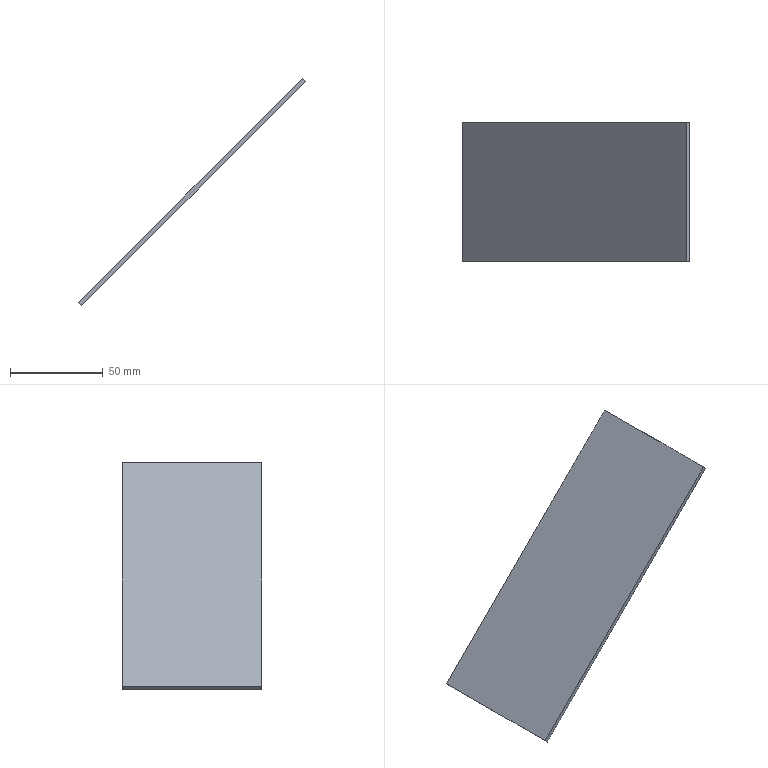Part | NX | features solid 2 | 1 solid | 6 faces | box 121.834 x 75.064 x 121.834 mm | volume 29350 mm3 | plane 6
STEP:
#1=CARTESIAN_POINT('',(-99.89,-600.064,-390.882));
#2=VERTEX_POINT('',#1);
#3=CARTESIAN_POINT('',(-98.264,-600.064,-392.508));
#4=VERTEX_POINT('',#3);
#5=CARTESIAN_POINT('',(-99.89,-600.064,-390.882));
#6=DIRECTION('',(-0.7071,0.,0.7071));
#7=VECTOR('',#6,1000.);
#8=LINE('',#5,#7);
#9=EDGE_CURVE('',#2,#4,#8,.F.);
#10=ORIENTED_EDGE('',*,*,#9,.F.);
#11=CARTESIAN_POINT('',(-99.89,-525.,-390.882));
#12=VERTEX_POINT('',#11);
#13=CARTESIAN_POINT('',(-99.89,-550.064,-390.882));
#14=DIRECTION('',(0.,1.,0.));
#15=VECTOR('',#14,1000.);
#16=LINE('',#13,#15);
#17=EDGE_CURVE('',#2,#12,#16,.T.);
#18=ORIENTED_EDGE('',*,*,#17,.T.);
#19=CARTESIAN_POINT('',(-98.264,-525.,-392.508));
#20=VERTEX_POINT('',#19);
#21=CARTESIAN_POINT('',(-99.89,-525.,-390.882));
#22=DIRECTION('',(0.7071,0.,-0.7071));
#23=VECTOR('',#22,1000.);
#24=LINE('',#21,#23);
#25=EDGE_CURVE('',#12,#20,#24,.T.);
#26=ORIENTED_EDGE('',*,*,#25,.T.);
#27=CARTESIAN_POINT('',(-98.264,-550.064,-392.508));
#28=DIRECTION('',(0.,1.,0.));
#29=VECTOR('',#28,1000.);
#30=LINE('',#27,#29);
#31=EDGE_CURVE('',#4,#20,#30,.T.);
#32=ORIENTED_EDGE('',*,*,#31,.F.);
#33=EDGE_LOOP('',(#10,#18,#26,#32));
#34=FACE_BOUND('',#33,.T.);
#35=CARTESIAN_POINT('',(-99.89,-550.064,-390.882));
#36=DIRECTION('',(-0.7071,0.,-0.7071));
#37=DIRECTION('',(0.,1.,0.));
#38=AXIS2_PLACEMENT_3D('',#35,#36,#37);
#39=PLANE('',#38);
#40=ADVANCED_FACE('',(#34),#39,.T.);
#41=ORIENTED_EDGE('',*,*,#25,.F.);
#42=CARTESIAN_POINT('',(20.318,-525.,-270.674));
#43=VERTEX_POINT('',#42);
#44=CARTESIAN_POINT('',(-50.393,-525.,-341.384));
#45=DIRECTION('',(0.7071,0.,0.7071));
#46=VECTOR('',#45,1000.);
#47=LINE('',#44,#46);
#48=EDGE_CURVE('',#12,#43,#47,.T.);
#49=ORIENTED_EDGE('',*,*,#48,.T.);
#50=CARTESIAN_POINT('',(21.944,-525.,-272.3));
#51=VERTEX_POINT('',#50);
#52=CARTESIAN_POINT('',(20.318,-525.,-270.674));
#53=DIRECTION('',(0.7071,0.,-0.7071));
#54=VECTOR('',#53,1000.);
#55=LINE('',#52,#54);
#56=EDGE_CURVE('',#43,#51,#55,.T.);
#57=ORIENTED_EDGE('',*,*,#56,.T.);
#58=CARTESIAN_POINT('',(-48.767,-525.,-343.011));
#59=DIRECTION('',(-0.7071,0.,-0.7071));
#60=VECTOR('',#59,1000.);
#61=LINE('',#58,#60);
#62=EDGE_CURVE('',#20,#51,#61,.F.);
#63=ORIENTED_EDGE('',*,*,#62,.F.);
#64=EDGE_LOOP('',(#41,#49,#57,#63));
#65=FACE_BOUND('',#64,.T.);
#66=CARTESIAN_POINT('',(-50.393,-525.,-341.384));
#67=DIRECTION('',(0.,1.,0.));
#68=DIRECTION('',(0.7071,0.,0.7071));
#69=AXIS2_PLACEMENT_3D('',#66,#67,#68);
#70=PLANE('',#69);
#71=ADVANCED_FACE('',(#65),#70,.T.);
#72=ORIENTED_EDGE('',*,*,#56,.F.);
#73=CARTESIAN_POINT('',(20.318,-600.064,-270.674));
#74=VERTEX_POINT('',#73);
#75=CARTESIAN_POINT('',(20.318,-550.064,-270.674));
#76=DIRECTION('',(0.,1.,0.));
#77=VECTOR('',#76,1000.);
#78=LINE('',#75,#77);
#79=EDGE_CURVE('',#74,#43,#78,.T.);
#80=ORIENTED_EDGE('',*,*,#79,.F.);
#81=CARTESIAN_POINT('',(21.944,-600.064,-272.3));
#82=VERTEX_POINT('',#81);
#83=CARTESIAN_POINT('',(20.318,-600.064,-270.674));
#84=DIRECTION('',(0.7071,0.,-0.7071));
#85=VECTOR('',#84,1000.);
#86=LINE('',#83,#85);
#87=EDGE_CURVE('',#74,#82,#86,.T.);
#88=ORIENTED_EDGE('',*,*,#87,.T.);
#89=CARTESIAN_POINT('',(21.944,-550.064,-272.3));
#90=DIRECTION('',(0.,1.,0.));
#91=VECTOR('',#90,1000.);
#92=LINE('',#89,#91);
#93=EDGE_CURVE('',#82,#51,#92,.T.);
#94=ORIENTED_EDGE('',*,*,#93,.T.);
#95=EDGE_LOOP('',(#72,#80,#88,#94));
#96=FACE_BOUND('',#95,.T.);
#97=CARTESIAN_POINT('',(20.318,-550.064,-270.674));
#98=DIRECTION('',(-0.7071,0.,-0.7071));
#99=DIRECTION('',(0.,1.,0.));
#100=AXIS2_PLACEMENT_3D('',#97,#98,#99);
#101=PLANE('',#100);
#102=ADVANCED_FACE('',(#96),#101,.F.);
#103=ORIENTED_EDGE('',*,*,#93,.F.);
#104=CARTESIAN_POINT('',(-48.767,-600.064,-343.011));
#105=DIRECTION('',(-0.7071,0.,-0.7071));
#106=VECTOR('',#105,1000.);
#107=LINE('',#104,#106);
#108=EDGE_CURVE('',#4,#82,#107,.F.);
#109=ORIENTED_EDGE('',*,*,#108,.F.);
#110=ORIENTED_EDGE('',*,*,#31,.T.);
#111=ORIENTED_EDGE('',*,*,#62,.T.);
#112=EDGE_LOOP('',(#103,#109,#110,#111));
#113=FACE_BOUND('',#112,.T.);
#114=CARTESIAN_POINT('',(-48.767,-550.064,-343.011));
#115=DIRECTION('',(0.7071,0.,-0.7071));
#116=DIRECTION('',(-0.7071,0.,-0.7071));
#117=AXIS2_PLACEMENT_3D('',#114,#115,#116);
#118=PLANE('',#117);
#119=ADVANCED_FACE('',(#113),#118,.T.);
#120=CARTESIAN_POINT('',(-50.393,-600.064,-341.384));
#121=DIRECTION('',(-0.7071,0.,-0.7071));
#122=VECTOR('',#121,1000.);
#123=LINE('',#120,#122);
#124=EDGE_CURVE('',#2,#74,#123,.F.);
#125=ORIENTED_EDGE('',*,*,#124,.F.);
#126=ORIENTED_EDGE('',*,*,#9,.T.);
#127=ORIENTED_EDGE('',*,*,#108,.T.);
#128=ORIENTED_EDGE('',*,*,#87,.F.);
#129=EDGE_LOOP('',(#125,#126,#127,#128));
#130=FACE_BOUND('',#129,.T.);
#131=CARTESIAN_POINT('',(-50.393,-600.064,-341.384));
#132=DIRECTION('',(0.,1.,0.));
#133=DIRECTION('',(0.7071,0.,0.7071));
#134=AXIS2_PLACEMENT_3D('',#131,#132,#133);
#135=PLANE('',#134);
#136=ADVANCED_FACE('',(#130),#135,.F.);
#137=ORIENTED_EDGE('',*,*,#79,.T.);
#138=ORIENTED_EDGE('',*,*,#48,.F.);
#139=ORIENTED_EDGE('',*,*,#17,.F.);
#140=ORIENTED_EDGE('',*,*,#124,.T.);
#141=EDGE_LOOP('',(#137,#138,#139,#140));
#142=FACE_BOUND('',#141,.T.);
#143=CARTESIAN_POINT('',(-50.393,-550.064,-341.384));
#144=DIRECTION('',(0.7071,0.,-0.7071));
#145=DIRECTION('',(-0.7071,0.,-0.7071));
#146=AXIS2_PLACEMENT_3D('',#143,#144,#145);
#147=PLANE('',#146);
#148=ADVANCED_FACE('',(#142),#147,.F.);
#149=CLOSED_SHELL('',(#40,#71,#102,#119,#136,#148));
#150=MANIFOLD_SOLID_BREP('',#149);
#151=(LENGTH_UNIT()NAMED_UNIT(*)SI_UNIT(.MILLI.,.METRE.));
#152=UNCERTAINTY_MEASURE_WITH_UNIT(LENGTH_MEASURE(0.00001),#151,'','');
#153=(NAMED_UNIT(*)PLANE_ANGLE_UNIT()SI_UNIT($,.RADIAN.));
#154=(NAMED_UNIT(*)SI_UNIT($,.STERADIAN.)SOLID_ANGLE_UNIT());
#155=(GEOMETRIC_REPRESENTATION_CONTEXT(3)GLOBAL_UNCERTAINTY_ASSIGNED_CONTEXT((#152))GLOBAL_UNIT_ASSIGNED_CONTEXT((#151,#153,#154))REPRESENTATION_CONTEXT('',''));
#156=ADVANCED_BREP_SHAPE_REPRESENTATION('',(#150),#155);